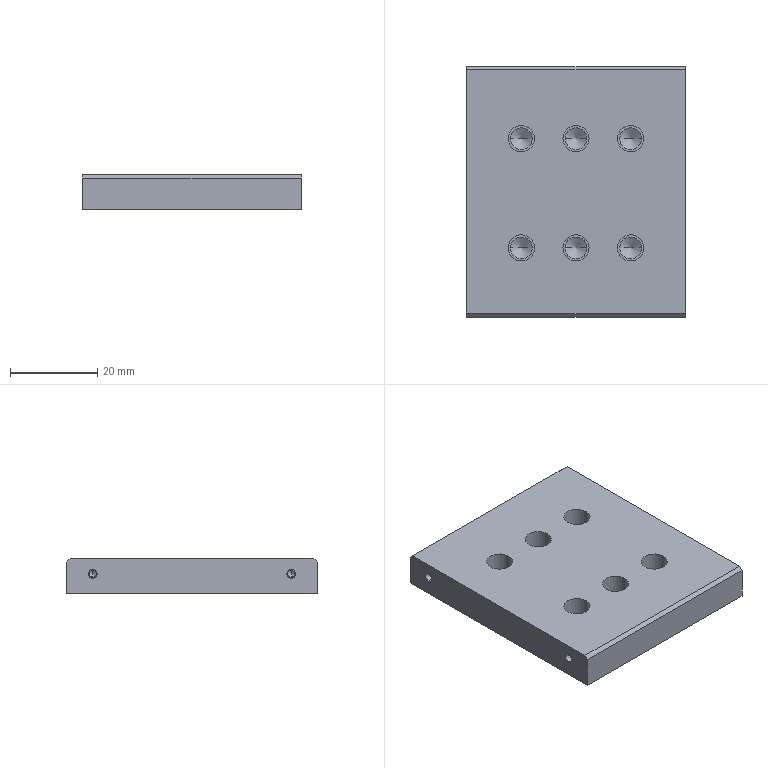Part | STEP file | ASND-0110-OPT-CO60-X-V1.0 front cover plate | 1 solid | 78 faces | box 50 x 57.4 x 8 mm | volume 21783 mm3 | cylinder 40 | cone 20 | plane 18 | commonest cylinder face diameters 5 x12 6 x12 1.6 x8 2 x8